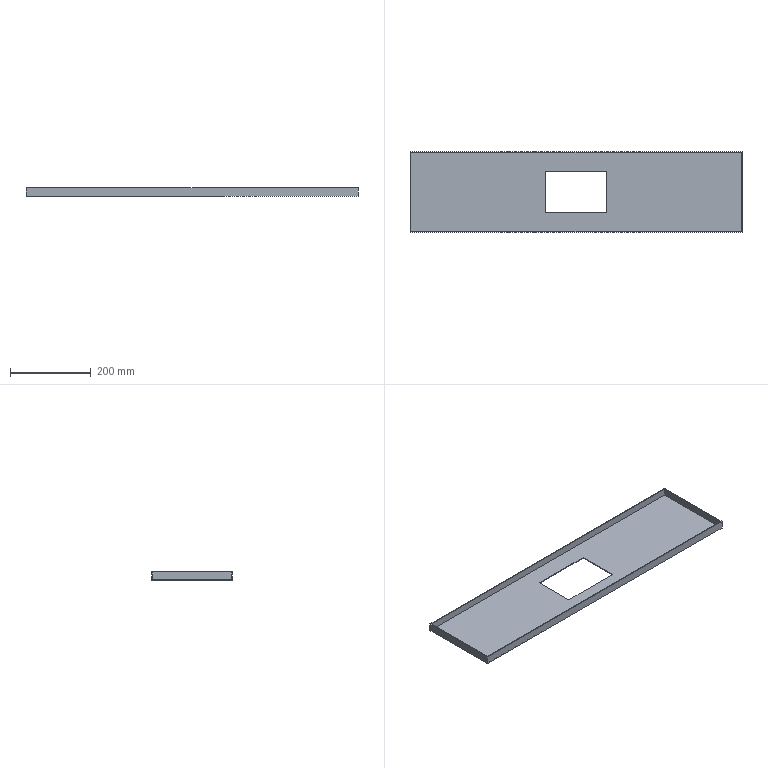Part | SolidWorks | features BaseBody 1 | 1 solid | 15 faces | box 820 x 200 x 20 mm | volume 369634 mm3 | plane 15
STEP:
#1=CARTESIAN_POINT('',(410.,-100.,-20.));
#2=VERTEX_POINT('',#1);
#3=CARTESIAN_POINT('',(410.,100.,-20.));
#4=VERTEX_POINT('',#3);
#5=CARTESIAN_POINT('',(410.,0.,-20.));
#6=DIRECTION('',(0.,1.,0.));
#7=VECTOR('',#6,1000.);
#8=LINE('',#5,#7);
#9=EDGE_CURVE('',#2,#4,#8,.T.);
#10=ORIENTED_EDGE('',*,*,#9,.T.);
#11=CARTESIAN_POINT('',(410.,100.,0.));
#12=VERTEX_POINT('',#11);
#13=CARTESIAN_POINT('',(410.,100.,-10.));
#14=DIRECTION('',(0.,0.,1.));
#15=VECTOR('',#14,1000.);
#16=LINE('',#13,#15);
#17=EDGE_CURVE('',#4,#12,#16,.T.);
#18=ORIENTED_EDGE('',*,*,#17,.T.);
#19=CARTESIAN_POINT('',(410.,-100.,0.));
#20=VERTEX_POINT('',#19);
#21=CARTESIAN_POINT('',(410.,0.,0.));
#22=DIRECTION('',(0.,-1.,0.));
#23=VECTOR('',#22,1000.);
#24=LINE('',#21,#23);
#25=EDGE_CURVE('',#12,#20,#24,.T.);
#26=ORIENTED_EDGE('',*,*,#25,.T.);
#27=CARTESIAN_POINT('',(410.,-100.,-10.));
#28=DIRECTION('',(0.,0.,-1.));
#29=VECTOR('',#28,1000.);
#30=LINE('',#27,#29);
#31=EDGE_CURVE('',#20,#2,#30,.T.);
#32=ORIENTED_EDGE('',*,*,#31,.T.);
#33=EDGE_LOOP('',(#10,#18,#26,#32));
#34=FACE_OUTER_BOUND('',#33,.T.);
#35=CARTESIAN_POINT('',(410.,-100.,0.));
#36=DIRECTION('',(1.,0.,0.));
#37=DIRECTION('',(0.,0.,-1.));
#38=AXIS2_PLACEMENT_3D('',#35,#36,#37);
#39=PLANE('',#38);
#40=ADVANCED_FACE('',(#34),#39,.T.);
#41=CARTESIAN_POINT('',(-410.,100.,-20.));
#42=VERTEX_POINT('',#41);
#43=CARTESIAN_POINT('',(0.,100.,-20.));
#44=DIRECTION('',(-1.,0.,0.));
#45=VECTOR('',#44,1000.);
#46=LINE('',#43,#45);
#47=EDGE_CURVE('',#4,#42,#46,.T.);
#48=ORIENTED_EDGE('',*,*,#47,.T.);
#49=CARTESIAN_POINT('',(-410.,100.,0.));
#50=VERTEX_POINT('',#49);
#51=CARTESIAN_POINT('',(-410.,100.,-10.));
#52=DIRECTION('',(0.,0.,1.));
#53=VECTOR('',#52,1000.);
#54=LINE('',#51,#53);
#55=EDGE_CURVE('',#42,#50,#54,.T.);
#56=ORIENTED_EDGE('',*,*,#55,.T.);
#57=CARTESIAN_POINT('',(0.,100.,0.));
#58=DIRECTION('',(1.,0.,0.));
#59=VECTOR('',#58,1000.);
#60=LINE('',#57,#59);
#61=EDGE_CURVE('',#50,#12,#60,.T.);
#62=ORIENTED_EDGE('',*,*,#61,.T.);
#63=ORIENTED_EDGE('',*,*,#17,.F.);
#64=EDGE_LOOP('',(#48,#56,#62,#63));
#65=FACE_OUTER_BOUND('',#64,.T.);
#66=CARTESIAN_POINT('',(-410.,100.,-20.));
#67=DIRECTION('',(0.,1.,0.));
#68=DIRECTION('',(0.,0.,1.));
#69=AXIS2_PLACEMENT_3D('',#66,#67,#68);
#70=PLANE('',#69);
#71=ADVANCED_FACE('',(#65),#70,.T.);
#72=CARTESIAN_POINT('',(76.5,-51.5,-20.));
#73=VERTEX_POINT('',#72);
#74=CARTESIAN_POINT('',(76.5,51.5,-20.));
#75=VERTEX_POINT('',#74);
#76=CARTESIAN_POINT('',(76.5,0.,-20.));
#77=DIRECTION('',(0.,1.,0.));
#78=VECTOR('',#77,1000.);
#79=LINE('',#76,#78);
#80=EDGE_CURVE('',#73,#75,#79,.T.);
#81=ORIENTED_EDGE('',*,*,#80,.T.);
#82=CARTESIAN_POINT('',(-76.5,51.5,-20.));
#83=VERTEX_POINT('',#82);
#84=CARTESIAN_POINT('',(0.,51.5,-20.));
#85=DIRECTION('',(-1.,0.,0.));
#86=VECTOR('',#85,1000.);
#87=LINE('',#84,#86);
#88=EDGE_CURVE('',#75,#83,#87,.T.);
#89=ORIENTED_EDGE('',*,*,#88,.T.);
#90=CARTESIAN_POINT('',(-76.5,-51.5,-20.));
#91=VERTEX_POINT('',#90);
#92=CARTESIAN_POINT('',(-76.5,0.,-20.));
#93=DIRECTION('',(0.,-1.,0.));
#94=VECTOR('',#93,1000.);
#95=LINE('',#92,#94);
#96=EDGE_CURVE('',#83,#91,#95,.T.);
#97=ORIENTED_EDGE('',*,*,#96,.T.);
#98=CARTESIAN_POINT('',(0.,-51.5,-20.));
#99=DIRECTION('',(1.,0.,0.));
#100=VECTOR('',#99,1000.);
#101=LINE('',#98,#100);
#102=EDGE_CURVE('',#91,#73,#101,.T.);
#103=ORIENTED_EDGE('',*,*,#102,.T.);
#104=EDGE_LOOP('',(#81,#89,#97,#103));
#105=FACE_BOUND('',#104,.T.);
#106=CARTESIAN_POINT('',(-410.,-100.,-20.));
#107=VERTEX_POINT('',#106);
#108=CARTESIAN_POINT('',(-410.,0.,-20.));
#109=DIRECTION('',(0.,1.,0.));
#110=VECTOR('',#109,1000.);
#111=LINE('',#108,#110);
#112=EDGE_CURVE('',#107,#42,#111,.T.);
#113=ORIENTED_EDGE('',*,*,#112,.T.);
#114=ORIENTED_EDGE('',*,*,#47,.F.);
#115=ORIENTED_EDGE('',*,*,#9,.F.);
#116=CARTESIAN_POINT('',(0.,-100.,-20.));
#117=DIRECTION('',(-1.,0.,0.));
#118=VECTOR('',#117,1000.);
#119=LINE('',#116,#118);
#120=EDGE_CURVE('',#2,#107,#119,.T.);
#121=ORIENTED_EDGE('',*,*,#120,.T.);
#122=EDGE_LOOP('',(#113,#114,#115,#121));
#123=FACE_OUTER_BOUND('',#122,.T.);
#124=CARTESIAN_POINT('',(410.,-100.,-20.));
#125=DIRECTION('',(0.,0.,-1.));
#126=DIRECTION('',(-1.,0.,0.));
#127=AXIS2_PLACEMENT_3D('',#124,#125,#126);
#128=PLANE('',#127);
#129=ADVANCED_FACE('',(#105,#123),#128,.T.);
#130=ORIENTED_EDGE('',*,*,#120,.F.);
#131=ORIENTED_EDGE('',*,*,#31,.F.);
#132=CARTESIAN_POINT('',(-410.,-100.,0.));
#133=VERTEX_POINT('',#132);
#134=CARTESIAN_POINT('',(0.,-100.,0.));
#135=DIRECTION('',(-1.,0.,0.));
#136=VECTOR('',#135,1000.);
#137=LINE('',#134,#136);
#138=EDGE_CURVE('',#20,#133,#137,.T.);
#139=ORIENTED_EDGE('',*,*,#138,.T.);
#140=CARTESIAN_POINT('',(-410.,-100.,-10.));
#141=DIRECTION('',(0.,0.,-1.));
#142=VECTOR('',#141,1000.);
#143=LINE('',#140,#142);
#144=EDGE_CURVE('',#133,#107,#143,.T.);
#145=ORIENTED_EDGE('',*,*,#144,.T.);
#146=EDGE_LOOP('',(#130,#131,#139,#145));
#147=FACE_OUTER_BOUND('',#146,.T.);
#148=CARTESIAN_POINT('',(-410.,-100.,0.));
#149=DIRECTION('',(0.,-1.,0.));
#150=DIRECTION('',(0.,0.,-1.));
#151=AXIS2_PLACEMENT_3D('',#148,#149,#150);
#152=PLANE('',#151);
#153=ADVANCED_FACE('',(#147),#152,.T.);
#154=CARTESIAN_POINT('',(-408.,98.,0.));
#155=VERTEX_POINT('',#154);
#156=CARTESIAN_POINT('',(-408.,-98.,0.));
#157=VERTEX_POINT('',#156);
#158=CARTESIAN_POINT('',(-408.,0.,0.));
#159=DIRECTION('',(0.,-1.,0.));
#160=VECTOR('',#159,1000.);
#161=LINE('',#158,#160);
#162=EDGE_CURVE('',#155,#157,#161,.T.);
#163=ORIENTED_EDGE('',*,*,#162,.F.);
#164=CARTESIAN_POINT('',(408.,98.,0.));
#165=VERTEX_POINT('',#164);
#166=CARTESIAN_POINT('',(0.,98.,0.));
#167=DIRECTION('',(-1.,0.,0.));
#168=VECTOR('',#167,1000.);
#169=LINE('',#166,#168);
#170=EDGE_CURVE('',#165,#155,#169,.T.);
#171=ORIENTED_EDGE('',*,*,#170,.F.);
#172=CARTESIAN_POINT('',(408.,-98.,0.));
#173=VERTEX_POINT('',#172);
#174=CARTESIAN_POINT('',(408.,0.,0.));
#175=DIRECTION('',(0.,1.,0.));
#176=VECTOR('',#175,1000.);
#177=LINE('',#174,#176);
#178=EDGE_CURVE('',#173,#165,#177,.T.);
#179=ORIENTED_EDGE('',*,*,#178,.F.);
#180=CARTESIAN_POINT('',(0.,-98.,0.));
#181=DIRECTION('',(1.,0.,0.));
#182=VECTOR('',#181,1000.);
#183=LINE('',#180,#182);
#184=EDGE_CURVE('',#157,#173,#183,.T.);
#185=ORIENTED_EDGE('',*,*,#184,.F.);
#186=EDGE_LOOP('',(#163,#171,#179,#185));
#187=FACE_BOUND('',#186,.T.);
#188=ORIENTED_EDGE('',*,*,#61,.F.);
#189=CARTESIAN_POINT('',(-410.,0.,0.));
#190=DIRECTION('',(0.,1.,0.));
#191=VECTOR('',#190,1000.);
#192=LINE('',#189,#191);
#193=EDGE_CURVE('',#133,#50,#192,.T.);
#194=ORIENTED_EDGE('',*,*,#193,.F.);
#195=ORIENTED_EDGE('',*,*,#138,.F.);
#196=ORIENTED_EDGE('',*,*,#25,.F.);
#197=EDGE_LOOP('',(#188,#194,#195,#196));
#198=FACE_OUTER_BOUND('',#197,.T.);
#199=CARTESIAN_POINT('',(410.,-100.,0.));
#200=DIRECTION('',(0.,0.,-1.));
#201=DIRECTION('',(-1.,0.,0.));
#202=AXIS2_PLACEMENT_3D('',#199,#200,#201);
#203=PLANE('',#202);
#204=ADVANCED_FACE('',(#187,#198),#203,.F.);
#205=ORIENTED_EDGE('',*,*,#112,.F.);
#206=ORIENTED_EDGE('',*,*,#144,.F.);
#207=ORIENTED_EDGE('',*,*,#193,.T.);
#208=ORIENTED_EDGE('',*,*,#55,.F.);
#209=EDGE_LOOP('',(#205,#206,#207,#208));
#210=FACE_OUTER_BOUND('',#209,.T.);
#211=CARTESIAN_POINT('',(-410.,-100.,-20.));
#212=DIRECTION('',(-1.,0.,0.));
#213=DIRECTION('',(0.,0.,1.));
#214=AXIS2_PLACEMENT_3D('',#211,#212,#213);
#215=PLANE('',#214);
#216=ADVANCED_FACE('',(#210),#215,.T.);
#217=CARTESIAN_POINT('',(-76.5,51.5,-18.));
#218=VERTEX_POINT('',#217);
#219=CARTESIAN_POINT('',(-76.5,51.5,-19.));
#220=DIRECTION('',(0.,0.,1.));
#221=VECTOR('',#220,1000.);
#222=LINE('',#219,#221);
#223=EDGE_CURVE('',#83,#218,#222,.T.);
#224=ORIENTED_EDGE('',*,*,#223,.F.);
#225=ORIENTED_EDGE('',*,*,#88,.F.);
#226=CARTESIAN_POINT('',(76.5,51.5,-18.));
#227=VERTEX_POINT('',#226);
#228=CARTESIAN_POINT('',(76.5,51.5,-19.));
#229=DIRECTION('',(0.,0.,-1.));
#230=VECTOR('',#229,1000.);
#231=LINE('',#228,#230);
#232=EDGE_CURVE('',#227,#75,#231,.T.);
#233=ORIENTED_EDGE('',*,*,#232,.F.);
#234=CARTESIAN_POINT('',(0.,51.5,-18.));
#235=DIRECTION('',(1.,0.,0.));
#236=VECTOR('',#235,1000.);
#237=LINE('',#234,#236);
#238=EDGE_CURVE('',#218,#227,#237,.T.);
#239=ORIENTED_EDGE('',*,*,#238,.F.);
#240=EDGE_LOOP('',(#224,#225,#233,#239));
#241=FACE_OUTER_BOUND('',#240,.T.);
#242=CARTESIAN_POINT('',(-76.5,51.5,-20.));
#243=DIRECTION('',(0.,1.,0.));
#244=DIRECTION('',(0.,0.,1.));
#245=AXIS2_PLACEMENT_3D('',#242,#243,#244);
#246=PLANE('',#245);
#247=ADVANCED_FACE('',(#241),#246,.F.);
#248=ORIENTED_EDGE('',*,*,#232,.T.);
#249=ORIENTED_EDGE('',*,*,#80,.F.);
#250=CARTESIAN_POINT('',(76.5,-51.5,-18.));
#251=VERTEX_POINT('',#250);
#252=CARTESIAN_POINT('',(76.5,-51.5,-19.));
#253=DIRECTION('',(0.,0.,-1.));
#254=VECTOR('',#253,1000.);
#255=LINE('',#252,#254);
#256=EDGE_CURVE('',#251,#73,#255,.T.);
#257=ORIENTED_EDGE('',*,*,#256,.F.);
#258=CARTESIAN_POINT('',(76.5,0.,-18.));
#259=DIRECTION('',(0.,-1.,0.));
#260=VECTOR('',#259,1000.);
#261=LINE('',#258,#260);
#262=EDGE_CURVE('',#227,#251,#261,.T.);
#263=ORIENTED_EDGE('',*,*,#262,.F.);
#264=EDGE_LOOP('',(#248,#249,#257,#263));
#265=FACE_OUTER_BOUND('',#264,.T.);
#266=CARTESIAN_POINT('',(76.5,-51.5,-18.));
#267=DIRECTION('',(1.,0.,0.));
#268=DIRECTION('',(0.,0.,-1.));
#269=AXIS2_PLACEMENT_3D('',#266,#267,#268);
#270=PLANE('',#269);
#271=ADVANCED_FACE('',(#265),#270,.F.);
#272=ORIENTED_EDGE('',*,*,#256,.T.);
#273=ORIENTED_EDGE('',*,*,#102,.F.);
#274=CARTESIAN_POINT('',(-76.5,-51.5,-18.));
#275=VERTEX_POINT('',#274);
#276=CARTESIAN_POINT('',(-76.5,-51.5,-19.));
#277=DIRECTION('',(0.,0.,-1.));
#278=VECTOR('',#277,1000.);
#279=LINE('',#276,#278);
#280=EDGE_CURVE('',#275,#91,#279,.T.);
#281=ORIENTED_EDGE('',*,*,#280,.F.);
#282=CARTESIAN_POINT('',(0.,-51.5,-18.));
#283=DIRECTION('',(-1.,0.,0.));
#284=VECTOR('',#283,1000.);
#285=LINE('',#282,#284);
#286=EDGE_CURVE('',#251,#275,#285,.T.);
#287=ORIENTED_EDGE('',*,*,#286,.F.);
#288=EDGE_LOOP('',(#272,#273,#281,#287));
#289=FACE_OUTER_BOUND('',#288,.T.);
#290=CARTESIAN_POINT('',(-76.5,-51.5,-18.));
#291=DIRECTION('',(0.,-1.,0.));
#292=DIRECTION('',(0.,0.,-1.));
#293=AXIS2_PLACEMENT_3D('',#290,#291,#292);
#294=PLANE('',#293);
#295=ADVANCED_FACE('',(#289),#294,.F.);
#296=ORIENTED_EDGE('',*,*,#280,.T.);
#297=ORIENTED_EDGE('',*,*,#96,.F.);
#298=ORIENTED_EDGE('',*,*,#223,.T.);
#299=CARTESIAN_POINT('',(-76.5,0.,-18.));
#300=DIRECTION('',(0.,1.,0.));
#301=VECTOR('',#300,1000.);
#302=LINE('',#299,#301);
#303=EDGE_CURVE('',#275,#218,#302,.T.);
#304=ORIENTED_EDGE('',*,*,#303,.F.);
#305=EDGE_LOOP('',(#296,#297,#298,#304));
#306=FACE_OUTER_BOUND('',#305,.T.);
#307=CARTESIAN_POINT('',(-76.5,-51.5,-20.));
#308=DIRECTION('',(-1.,0.,0.));
#309=DIRECTION('',(0.,0.,1.));
#310=AXIS2_PLACEMENT_3D('',#307,#308,#309);
#311=PLANE('',#310);
#312=ADVANCED_FACE('',(#306),#311,.F.);
#313=CARTESIAN_POINT('',(408.,-98.,-18.));
#314=VERTEX_POINT('',#313);
#315=CARTESIAN_POINT('',(408.,-98.,-9.));
#316=DIRECTION('',(0.,0.,1.));
#317=VECTOR('',#316,1000.);
#318=LINE('',#315,#317);
#319=EDGE_CURVE('',#314,#173,#318,.T.);
#320=ORIENTED_EDGE('',*,*,#319,.F.);
#321=CARTESIAN_POINT('',(-408.,-98.,-18.));
#322=VERTEX_POINT('',#321);
#323=CARTESIAN_POINT('',(0.,-98.,-18.));
#324=DIRECTION('',(1.,0.,0.));
#325=VECTOR('',#324,1000.);
#326=LINE('',#323,#325);
#327=EDGE_CURVE('',#322,#314,#326,.T.);
#328=ORIENTED_EDGE('',*,*,#327,.F.);
#329=CARTESIAN_POINT('',(-408.,-98.,-9.));
#330=DIRECTION('',(0.,0.,-1.));
#331=VECTOR('',#330,1000.);
#332=LINE('',#329,#331);
#333=EDGE_CURVE('',#157,#322,#332,.T.);
#334=ORIENTED_EDGE('',*,*,#333,.F.);
#335=ORIENTED_EDGE('',*,*,#184,.T.);
#336=EDGE_LOOP('',(#320,#328,#334,#335));
#337=FACE_OUTER_BOUND('',#336,.T.);
#338=CARTESIAN_POINT('',(-408.,-98.,-18.));
#339=DIRECTION('',(0.,-1.,0.));
#340=DIRECTION('',(1.,0.,0.));
#341=AXIS2_PLACEMENT_3D('',#338,#339,#340);
#342=PLANE('',#341);
#343=ADVANCED_FACE('',(#337),#342,.F.);
#344=ORIENTED_EDGE('',*,*,#333,.T.);
#345=CARTESIAN_POINT('',(-408.,98.,-18.));
#346=VERTEX_POINT('',#345);
#347=CARTESIAN_POINT('',(-408.,0.,-18.));
#348=DIRECTION('',(0.,-1.,0.));
#349=VECTOR('',#348,1000.);
#350=LINE('',#347,#349);
#351=EDGE_CURVE('',#346,#322,#350,.T.);
#352=ORIENTED_EDGE('',*,*,#351,.F.);
#353=CARTESIAN_POINT('',(-408.,98.,-9.));
#354=DIRECTION('',(0.,0.,-1.));
#355=VECTOR('',#354,1000.);
#356=LINE('',#353,#355);
#357=EDGE_CURVE('',#155,#346,#356,.T.);
#358=ORIENTED_EDGE('',*,*,#357,.F.);
#359=ORIENTED_EDGE('',*,*,#162,.T.);
#360=EDGE_LOOP('',(#344,#352,#358,#359));
#361=FACE_OUTER_BOUND('',#360,.T.);
#362=CARTESIAN_POINT('',(-408.,-98.,-18.));
#363=DIRECTION('',(-1.,0.,0.));
#364=DIRECTION('',(0.,0.,1.));
#365=AXIS2_PLACEMENT_3D('',#362,#363,#364);
#366=PLANE('',#365);
#367=ADVANCED_FACE('',(#361),#366,.F.);
#368=ORIENTED_EDGE('',*,*,#357,.T.);
#369=CARTESIAN_POINT('',(408.,98.,-18.));
#370=VERTEX_POINT('',#369);
#371=CARTESIAN_POINT('',(0.,98.,-18.));
#372=DIRECTION('',(-1.,0.,0.));
#373=VECTOR('',#372,1000.);
#374=LINE('',#371,#373);
#375=EDGE_CURVE('',#370,#346,#374,.T.);
#376=ORIENTED_EDGE('',*,*,#375,.F.);
#377=CARTESIAN_POINT('',(408.,98.,-9.));
#378=DIRECTION('',(0.,0.,-1.));
#379=VECTOR('',#378,1000.);
#380=LINE('',#377,#379);
#381=EDGE_CURVE('',#165,#370,#380,.T.);
#382=ORIENTED_EDGE('',*,*,#381,.F.);
#383=ORIENTED_EDGE('',*,*,#170,.T.);
#384=EDGE_LOOP('',(#368,#376,#382,#383));
#385=FACE_OUTER_BOUND('',#384,.T.);
#386=CARTESIAN_POINT('',(408.,98.,-18.));
#387=DIRECTION('',(0.,1.,0.));
#388=DIRECTION('',(-1.,0.,0.));
#389=AXIS2_PLACEMENT_3D('',#386,#387,#388);
#390=PLANE('',#389);
#391=ADVANCED_FACE('',(#385),#390,.F.);
#392=ORIENTED_EDGE('',*,*,#381,.T.);
#393=CARTESIAN_POINT('',(408.,0.,-18.));
#394=DIRECTION('',(0.,1.,0.));
#395=VECTOR('',#394,1000.);
#396=LINE('',#393,#395);
#397=EDGE_CURVE('',#314,#370,#396,.T.);
#398=ORIENTED_EDGE('',*,*,#397,.F.);
#399=ORIENTED_EDGE('',*,*,#319,.T.);
#400=ORIENTED_EDGE('',*,*,#178,.T.);
#401=EDGE_LOOP('',(#392,#398,#399,#400));
#402=FACE_OUTER_BOUND('',#401,.T.);
#403=CARTESIAN_POINT('',(408.,-98.,0.));
#404=DIRECTION('',(1.,0.,0.));
#405=DIRECTION('',(0.,0.,-1.));
#406=AXIS2_PLACEMENT_3D('',#403,#404,#405);
#407=PLANE('',#406);
#408=ADVANCED_FACE('',(#402),#407,.F.);
#409=ORIENTED_EDGE('',*,*,#262,.T.);
#410=ORIENTED_EDGE('',*,*,#286,.T.);
#411=ORIENTED_EDGE('',*,*,#303,.T.);
#412=ORIENTED_EDGE('',*,*,#238,.T.);
#413=EDGE_LOOP('',(#409,#410,#411,#412));
#414=FACE_BOUND('',#413,.T.);
#415=ORIENTED_EDGE('',*,*,#397,.T.);
#416=ORIENTED_EDGE('',*,*,#375,.T.);
#417=ORIENTED_EDGE('',*,*,#351,.T.);
#418=ORIENTED_EDGE('',*,*,#327,.T.);
#419=EDGE_LOOP('',(#415,#416,#417,#418));
#420=FACE_OUTER_BOUND('',#419,.T.);
#421=CARTESIAN_POINT('',(-408.,-98.,-18.));
#422=DIRECTION('',(0.,0.,1.));
#423=DIRECTION('',(1.,0.,0.));
#424=AXIS2_PLACEMENT_3D('',#421,#422,#423);
#425=PLANE('',#424);
#426=ADVANCED_FACE('',(#414,#420),#425,.T.);
#427=CLOSED_SHELL('',(#40,#71,#129,#153,#204,#216,#247,#271,#295,#312,#343,#367,#391,#408,#426));
#428=MANIFOLD_SOLID_BREP('',#427);
#429=CARTESIAN_POINT('',(0.,0.,0.));
#430=DIRECTION('',(0.,0.,1.));
#431=DIRECTION('',(1.,0.,0.));
#432=AXIS2_PLACEMENT_3D('',#429,#430,#431);
#433=(LENGTH_UNIT()NAMED_UNIT(*)SI_UNIT(.MILLI.,.METRE.));
#434=UNCERTAINTY_MEASURE_WITH_UNIT(LENGTH_MEASURE(0.00001),#433,'','');
#435=(NAMED_UNIT(*)PLANE_ANGLE_UNIT()SI_UNIT($,.RADIAN.));
#436=(NAMED_UNIT(*)SI_UNIT($,.STERADIAN.)SOLID_ANGLE_UNIT());
#437=(GEOMETRIC_REPRESENTATION_CONTEXT(3)GLOBAL_UNCERTAINTY_ASSIGNED_CONTEXT((#434))GLOBAL_UNIT_ASSIGNED_CONTEXT((#433,#435,#436))REPRESENTATION_CONTEXT('',''));
#438=ADVANCED_BREP_SHAPE_REPRESENTATION('',(#428,#432),#437);